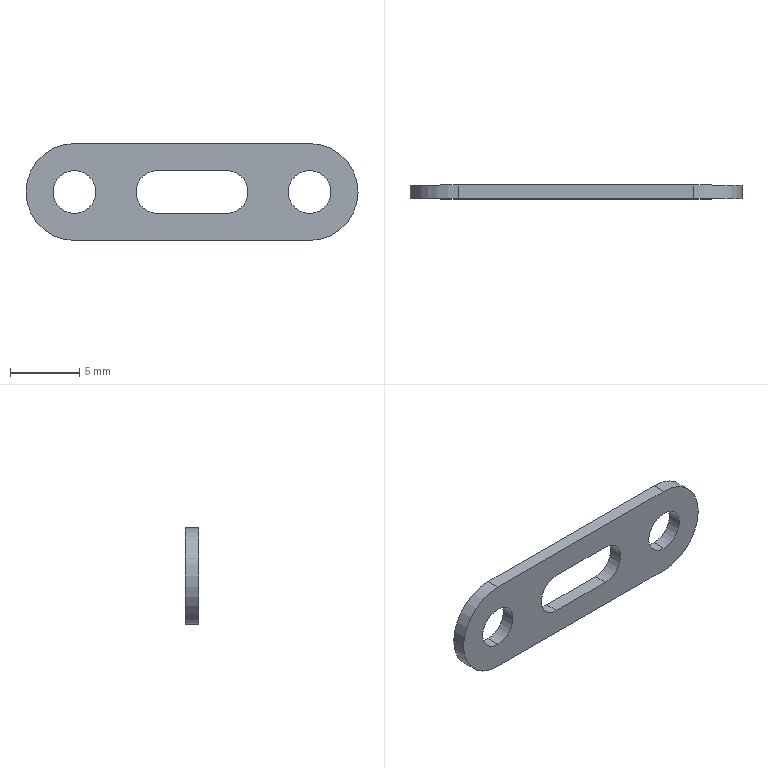Part | SolidWorks | features Extrusion 1 | 1 solid | 14 faces | box 23.98 x 1 x 7 mm | volume 119.201 mm3 | cylinder 8 | plane 6 | commonest cylinder face diameters 3.1 x6 7 x2
STEP:
#1=CARTESIAN_POINT('',(16.98,1.,-1.55));
#2=VERTEX_POINT('',#1);
#3=CARTESIAN_POINT('',(16.98,1.,1.55));
#4=VERTEX_POINT('',#3);
#5=CARTESIAN_POINT('',(16.98,1.,0.));
#6=DIRECTION('',(0.,1.,0.));
#7=DIRECTION('',(0.,0.,1.));
#8=AXIS2_PLACEMENT_3D('',#5,#6,#7);
#9=CIRCLE('',#8,1.55);
#10=EDGE_CURVE('',#2,#4,#9,.T.);
#11=ORIENTED_EDGE('',*,*,#10,.T.);
#12=CARTESIAN_POINT('',(16.98,0.,1.55));
#13=VERTEX_POINT('',#12);
#14=CARTESIAN_POINT('',(16.98,1.,1.55));
#15=DIRECTION('',(0.,-1.,0.));
#16=VECTOR('',#15,1000.);
#17=LINE('',#14,#16);
#18=EDGE_CURVE('',#4,#13,#17,.T.);
#19=ORIENTED_EDGE('',*,*,#18,.T.);
#20=CARTESIAN_POINT('',(16.98,0.,-1.55));
#21=VERTEX_POINT('',#20);
#22=CARTESIAN_POINT('',(16.98,0.,0.));
#23=DIRECTION('',(0.,1.,0.));
#24=DIRECTION('',(0.,0.,1.));
#25=AXIS2_PLACEMENT_3D('',#22,#23,#24);
#26=CIRCLE('',#25,1.55);
#27=EDGE_CURVE('',#21,#13,#26,.T.);
#28=ORIENTED_EDGE('',*,*,#27,.F.);
#29=CARTESIAN_POINT('',(16.98,1.,-1.55));
#30=DIRECTION('',(0.,-1.,0.));
#31=VECTOR('',#30,1000.);
#32=LINE('',#29,#31);
#33=EDGE_CURVE('',#2,#21,#32,.T.);
#34=ORIENTED_EDGE('',*,*,#33,.F.);
#35=EDGE_LOOP('',(#11,#19,#28,#34));
#36=FACE_OUTER_BOUND('',#35,.T.);
#37=CARTESIAN_POINT('',(16.98,1.,0.));
#38=DIRECTION('',(0.,-1.,0.));
#39=DIRECTION('',(0.,0.,-1.));
#40=AXIS2_PLACEMENT_3D('',#37,#38,#39);
#41=CYLINDRICAL_SURFACE('',#40,1.55);
#42=ADVANCED_FACE('',(#36),#41,.F.);
#43=CARTESIAN_POINT('',(0.,1.,-1.55));
#44=VERTEX_POINT('',#43);
#45=CARTESIAN_POINT('',(0.,1.,1.55));
#46=VERTEX_POINT('',#45);
#47=CARTESIAN_POINT('',(0.,1.,0.));
#48=DIRECTION('',(0.,1.,0.));
#49=DIRECTION('',(0.,0.,1.));
#50=AXIS2_PLACEMENT_3D('',#47,#48,#49);
#51=CIRCLE('',#50,1.55);
#52=EDGE_CURVE('',#44,#46,#51,.T.);
#53=ORIENTED_EDGE('',*,*,#52,.T.);
#54=CARTESIAN_POINT('',(0.,0.,1.55));
#55=VERTEX_POINT('',#54);
#56=CARTESIAN_POINT('',(0.,1.,1.55));
#57=DIRECTION('',(0.,-1.,0.));
#58=VECTOR('',#57,1000.);
#59=LINE('',#56,#58);
#60=EDGE_CURVE('',#46,#55,#59,.T.);
#61=ORIENTED_EDGE('',*,*,#60,.T.);
#62=CARTESIAN_POINT('',(0.,0.,-1.55));
#63=VERTEX_POINT('',#62);
#64=CARTESIAN_POINT('',(0.,0.,0.));
#65=DIRECTION('',(0.,1.,0.));
#66=DIRECTION('',(0.,0.,1.));
#67=AXIS2_PLACEMENT_3D('',#64,#65,#66);
#68=CIRCLE('',#67,1.55);
#69=EDGE_CURVE('',#63,#55,#68,.T.);
#70=ORIENTED_EDGE('',*,*,#69,.F.);
#71=CARTESIAN_POINT('',(0.,1.,-1.55));
#72=DIRECTION('',(0.,-1.,0.));
#73=VECTOR('',#72,1000.);
#74=LINE('',#71,#73);
#75=EDGE_CURVE('',#44,#63,#74,.T.);
#76=ORIENTED_EDGE('',*,*,#75,.F.);
#77=EDGE_LOOP('',(#53,#61,#70,#76));
#78=FACE_OUTER_BOUND('',#77,.T.);
#79=CARTESIAN_POINT('',(0.,1.,0.));
#80=DIRECTION('',(0.,-1.,0.));
#81=DIRECTION('',(0.,0.,-1.));
#82=AXIS2_PLACEMENT_3D('',#79,#80,#81);
#83=CYLINDRICAL_SURFACE('',#82,1.55);
#84=ADVANCED_FACE('',(#78),#83,.F.);
#85=CARTESIAN_POINT('',(10.99,0.,1.55));
#86=VERTEX_POINT('',#85);
#87=CARTESIAN_POINT('',(10.99,0.,-1.55));
#88=VERTEX_POINT('',#87);
#89=CARTESIAN_POINT('',(10.99,0.,0.));
#90=DIRECTION('',(0.,1.,0.));
#91=DIRECTION('',(0.,0.,1.));
#92=AXIS2_PLACEMENT_3D('',#89,#90,#91);
#93=CIRCLE('',#92,1.55);
#94=EDGE_CURVE('',#86,#88,#93,.T.);
#95=ORIENTED_EDGE('',*,*,#94,.F.);
#96=CARTESIAN_POINT('',(10.99,1.,1.55));
#97=VERTEX_POINT('',#96);
#98=CARTESIAN_POINT('',(10.99,1.,1.55));
#99=DIRECTION('',(0.,-1.,0.));
#100=VECTOR('',#99,1000.);
#101=LINE('',#98,#100);
#102=EDGE_CURVE('',#97,#86,#101,.T.);
#103=ORIENTED_EDGE('',*,*,#102,.F.);
#104=CARTESIAN_POINT('',(10.99,1.,-1.55));
#105=VERTEX_POINT('',#104);
#106=CARTESIAN_POINT('',(10.99,1.,0.));
#107=DIRECTION('',(0.,1.,0.));
#108=DIRECTION('',(0.,0.,1.));
#109=AXIS2_PLACEMENT_3D('',#106,#107,#108);
#110=CIRCLE('',#109,1.55);
#111=EDGE_CURVE('',#97,#105,#110,.T.);
#112=ORIENTED_EDGE('',*,*,#111,.T.);
#113=CARTESIAN_POINT('',(10.99,1.,-1.55));
#114=DIRECTION('',(0.,-1.,0.));
#115=VECTOR('',#114,1000.);
#116=LINE('',#113,#115);
#117=EDGE_CURVE('',#105,#88,#116,.T.);
#118=ORIENTED_EDGE('',*,*,#117,.T.);
#119=EDGE_LOOP('',(#95,#103,#112,#118));
#120=FACE_OUTER_BOUND('',#119,.T.);
#121=CARTESIAN_POINT('',(10.99,1.,0.));
#122=DIRECTION('',(0.,-1.,0.));
#123=DIRECTION('',(0.,0.,-1.));
#124=AXIS2_PLACEMENT_3D('',#121,#122,#123);
#125=CYLINDRICAL_SURFACE('',#124,1.55);
#126=ADVANCED_FACE('',(#120),#125,.F.);
#127=CARTESIAN_POINT('',(5.99,0.,1.55));
#128=VERTEX_POINT('',#127);
#129=CARTESIAN_POINT('',(0.,0.,1.55));
#130=DIRECTION('',(1.,0.,0.));
#131=VECTOR('',#130,1000.);
#132=LINE('',#129,#131);
#133=EDGE_CURVE('',#128,#86,#132,.T.);
#134=ORIENTED_EDGE('',*,*,#133,.F.);
#135=CARTESIAN_POINT('',(5.99,1.,1.55));
#136=VERTEX_POINT('',#135);
#137=CARTESIAN_POINT('',(5.99,1.,1.55));
#138=DIRECTION('',(0.,-1.,0.));
#139=VECTOR('',#138,1000.);
#140=LINE('',#137,#139);
#141=EDGE_CURVE('',#136,#128,#140,.T.);
#142=ORIENTED_EDGE('',*,*,#141,.F.);
#143=CARTESIAN_POINT('',(0.,1.,1.55));
#144=DIRECTION('',(1.,0.,0.));
#145=VECTOR('',#144,1000.);
#146=LINE('',#143,#145);
#147=EDGE_CURVE('',#136,#97,#146,.T.);
#148=ORIENTED_EDGE('',*,*,#147,.T.);
#149=ORIENTED_EDGE('',*,*,#102,.T.);
#150=EDGE_LOOP('',(#134,#142,#148,#149));
#151=FACE_OUTER_BOUND('',#150,.T.);
#152=CARTESIAN_POINT('',(0.,1.,1.55));
#153=DIRECTION('',(0.,0.,-1.));
#154=DIRECTION('',(-1.,0.,0.));
#155=AXIS2_PLACEMENT_3D('',#152,#153,#154);
#156=PLANE('',#155);
#157=ADVANCED_FACE('',(#151),#156,.T.);
#158=CARTESIAN_POINT('',(5.99,0.,-1.55));
#159=VERTEX_POINT('',#158);
#160=CARTESIAN_POINT('',(5.99,0.,0.));
#161=DIRECTION('',(0.,1.,0.));
#162=DIRECTION('',(0.,0.,1.));
#163=AXIS2_PLACEMENT_3D('',#160,#161,#162);
#164=CIRCLE('',#163,1.55);
#165=EDGE_CURVE('',#159,#128,#164,.T.);
#166=ORIENTED_EDGE('',*,*,#165,.F.);
#167=CARTESIAN_POINT('',(5.99,1.,-1.55));
#168=VERTEX_POINT('',#167);
#169=CARTESIAN_POINT('',(5.99,1.,-1.55));
#170=DIRECTION('',(0.,-1.,0.));
#171=VECTOR('',#170,1000.);
#172=LINE('',#169,#171);
#173=EDGE_CURVE('',#168,#159,#172,.T.);
#174=ORIENTED_EDGE('',*,*,#173,.F.);
#175=CARTESIAN_POINT('',(5.99,1.,0.));
#176=DIRECTION('',(0.,1.,0.));
#177=DIRECTION('',(0.,0.,1.));
#178=AXIS2_PLACEMENT_3D('',#175,#176,#177);
#179=CIRCLE('',#178,1.55);
#180=EDGE_CURVE('',#168,#136,#179,.T.);
#181=ORIENTED_EDGE('',*,*,#180,.T.);
#182=ORIENTED_EDGE('',*,*,#141,.T.);
#183=EDGE_LOOP('',(#166,#174,#181,#182));
#184=FACE_OUTER_BOUND('',#183,.T.);
#185=CARTESIAN_POINT('',(5.99,1.,0.));
#186=DIRECTION('',(0.,-1.,0.));
#187=DIRECTION('',(0.,0.,-1.));
#188=AXIS2_PLACEMENT_3D('',#185,#186,#187);
#189=CYLINDRICAL_SURFACE('',#188,1.55);
#190=ADVANCED_FACE('',(#184),#189,.F.);
#191=CARTESIAN_POINT('',(0.,0.,-3.5));
#192=VERTEX_POINT('',#191);
#193=CARTESIAN_POINT('',(0.,0.,3.5));
#194=VERTEX_POINT('',#193);
#195=CARTESIAN_POINT('',(0.,0.,0.));
#196=DIRECTION('',(0.,1.,0.));
#197=DIRECTION('',(0.,0.,1.));
#198=AXIS2_PLACEMENT_3D('',#195,#196,#197);
#199=CIRCLE('',#198,3.5);
#200=EDGE_CURVE('',#192,#194,#199,.T.);
#201=ORIENTED_EDGE('',*,*,#200,.T.);
#202=CARTESIAN_POINT('',(0.,1.,3.5));
#203=VERTEX_POINT('',#202);
#204=CARTESIAN_POINT('',(0.,1.,3.5));
#205=DIRECTION('',(0.,-1.,0.));
#206=VECTOR('',#205,1000.);
#207=LINE('',#204,#206);
#208=EDGE_CURVE('',#203,#194,#207,.T.);
#209=ORIENTED_EDGE('',*,*,#208,.F.);
#210=CARTESIAN_POINT('',(0.,1.,-3.5));
#211=VERTEX_POINT('',#210);
#212=CARTESIAN_POINT('',(0.,1.,0.));
#213=DIRECTION('',(0.,1.,0.));
#214=DIRECTION('',(0.,0.,1.));
#215=AXIS2_PLACEMENT_3D('',#212,#213,#214);
#216=CIRCLE('',#215,3.5);
#217=EDGE_CURVE('',#211,#203,#216,.T.);
#218=ORIENTED_EDGE('',*,*,#217,.F.);
#219=CARTESIAN_POINT('',(0.,1.,-3.5));
#220=DIRECTION('',(0.,-1.,0.));
#221=VECTOR('',#220,1000.);
#222=LINE('',#219,#221);
#223=EDGE_CURVE('',#211,#192,#222,.T.);
#224=ORIENTED_EDGE('',*,*,#223,.T.);
#225=EDGE_LOOP('',(#201,#209,#218,#224));
#226=FACE_OUTER_BOUND('',#225,.T.);
#227=CARTESIAN_POINT('',(0.,1.,0.));
#228=DIRECTION('',(0.,-1.,0.));
#229=DIRECTION('',(0.,0.,-1.));
#230=AXIS2_PLACEMENT_3D('',#227,#228,#229);
#231=CYLINDRICAL_SURFACE('',#230,3.5);
#232=ADVANCED_FACE('',(#226),#231,.T.);
#233=CARTESIAN_POINT('',(16.98,0.,3.5));
#234=VERTEX_POINT('',#233);
#235=CARTESIAN_POINT('',(0.,0.,3.5));
#236=DIRECTION('',(1.,0.,0.));
#237=VECTOR('',#236,1000.);
#238=LINE('',#235,#237);
#239=EDGE_CURVE('',#194,#234,#238,.T.);
#240=ORIENTED_EDGE('',*,*,#239,.T.);
#241=CARTESIAN_POINT('',(16.98,1.,3.5));
#242=VERTEX_POINT('',#241);
#243=CARTESIAN_POINT('',(16.98,1.,3.5));
#244=DIRECTION('',(0.,-1.,0.));
#245=VECTOR('',#244,1000.);
#246=LINE('',#243,#245);
#247=EDGE_CURVE('',#242,#234,#246,.T.);
#248=ORIENTED_EDGE('',*,*,#247,.F.);
#249=CARTESIAN_POINT('',(0.,1.,3.5));
#250=DIRECTION('',(1.,0.,0.));
#251=VECTOR('',#250,1000.);
#252=LINE('',#249,#251);
#253=EDGE_CURVE('',#203,#242,#252,.T.);
#254=ORIENTED_EDGE('',*,*,#253,.F.);
#255=ORIENTED_EDGE('',*,*,#208,.T.);
#256=EDGE_LOOP('',(#240,#248,#254,#255));
#257=FACE_OUTER_BOUND('',#256,.T.);
#258=CARTESIAN_POINT('',(0.,1.,3.5));
#259=DIRECTION('',(0.,0.,-1.));
#260=DIRECTION('',(-1.,0.,0.));
#261=AXIS2_PLACEMENT_3D('',#258,#259,#260);
#262=PLANE('',#261);
#263=ADVANCED_FACE('',(#257),#262,.F.);
#264=CARTESIAN_POINT('',(16.98,0.,-3.5));
#265=VERTEX_POINT('',#264);
#266=CARTESIAN_POINT('',(16.98,0.,0.));
#267=DIRECTION('',(0.,1.,0.));
#268=DIRECTION('',(0.,0.,1.));
#269=AXIS2_PLACEMENT_3D('',#266,#267,#268);
#270=CIRCLE('',#269,3.5);
#271=EDGE_CURVE('',#234,#265,#270,.T.);
#272=ORIENTED_EDGE('',*,*,#271,.T.);
#273=CARTESIAN_POINT('',(16.98,1.,-3.5));
#274=VERTEX_POINT('',#273);
#275=CARTESIAN_POINT('',(16.98,1.,-3.5));
#276=DIRECTION('',(0.,-1.,0.));
#277=VECTOR('',#276,1000.);
#278=LINE('',#275,#277);
#279=EDGE_CURVE('',#274,#265,#278,.T.);
#280=ORIENTED_EDGE('',*,*,#279,.F.);
#281=CARTESIAN_POINT('',(16.98,1.,0.));
#282=DIRECTION('',(0.,1.,0.));
#283=DIRECTION('',(0.,0.,1.));
#284=AXIS2_PLACEMENT_3D('',#281,#282,#283);
#285=CIRCLE('',#284,3.5);
#286=EDGE_CURVE('',#242,#274,#285,.T.);
#287=ORIENTED_EDGE('',*,*,#286,.F.);
#288=ORIENTED_EDGE('',*,*,#247,.T.);
#289=EDGE_LOOP('',(#272,#280,#287,#288));
#290=FACE_OUTER_BOUND('',#289,.T.);
#291=CARTESIAN_POINT('',(16.98,1.,0.));
#292=DIRECTION('',(0.,-1.,0.));
#293=DIRECTION('',(0.,0.,-1.));
#294=AXIS2_PLACEMENT_3D('',#291,#292,#293);
#295=CYLINDRICAL_SURFACE('',#294,3.5);
#296=ADVANCED_FACE('',(#290),#295,.T.);
#297=CARTESIAN_POINT('',(0.,0.,-1.55));
#298=DIRECTION('',(1.,0.,0.));
#299=VECTOR('',#298,1000.);
#300=LINE('',#297,#299);
#301=EDGE_CURVE('',#159,#88,#300,.T.);
#302=ORIENTED_EDGE('',*,*,#301,.T.);
#303=ORIENTED_EDGE('',*,*,#117,.F.);
#304=CARTESIAN_POINT('',(0.,1.,-1.55));
#305=DIRECTION('',(1.,0.,0.));
#306=VECTOR('',#305,1000.);
#307=LINE('',#304,#306);
#308=EDGE_CURVE('',#168,#105,#307,.T.);
#309=ORIENTED_EDGE('',*,*,#308,.F.);
#310=ORIENTED_EDGE('',*,*,#173,.T.);
#311=EDGE_LOOP('',(#302,#303,#309,#310));
#312=FACE_OUTER_BOUND('',#311,.T.);
#313=CARTESIAN_POINT('',(0.,1.,-1.55));
#314=DIRECTION('',(0.,0.,-1.));
#315=DIRECTION('',(-1.,0.,0.));
#316=AXIS2_PLACEMENT_3D('',#313,#314,#315);
#317=PLANE('',#316);
#318=ADVANCED_FACE('',(#312),#317,.F.);
#319=CARTESIAN_POINT('',(0.,0.,-3.5));
#320=DIRECTION('',(1.,0.,0.));
#321=VECTOR('',#320,1000.);
#322=LINE('',#319,#321);
#323=EDGE_CURVE('',#192,#265,#322,.T.);
#324=ORIENTED_EDGE('',*,*,#323,.F.);
#325=ORIENTED_EDGE('',*,*,#223,.F.);
#326=CARTESIAN_POINT('',(0.,1.,-3.5));
#327=DIRECTION('',(1.,0.,0.));
#328=VECTOR('',#327,1000.);
#329=LINE('',#326,#328);
#330=EDGE_CURVE('',#211,#274,#329,.T.);
#331=ORIENTED_EDGE('',*,*,#330,.T.);
#332=ORIENTED_EDGE('',*,*,#279,.T.);
#333=EDGE_LOOP('',(#324,#325,#331,#332));
#334=FACE_OUTER_BOUND('',#333,.T.);
#335=CARTESIAN_POINT('',(0.,1.,-3.5));
#336=DIRECTION('',(0.,0.,-1.));
#337=DIRECTION('',(-1.,0.,0.));
#338=AXIS2_PLACEMENT_3D('',#335,#336,#337);
#339=PLANE('',#338);
#340=ADVANCED_FACE('',(#334),#339,.T.);
#341=ORIENTED_EDGE('',*,*,#60,.F.);
#342=CARTESIAN_POINT('',(0.,1.,0.));
#343=DIRECTION('',(0.,1.,0.));
#344=DIRECTION('',(0.,0.,1.));
#345=AXIS2_PLACEMENT_3D('',#342,#343,#344);
#346=CIRCLE('',#345,1.55);
#347=EDGE_CURVE('',#46,#44,#346,.T.);
#348=ORIENTED_EDGE('',*,*,#347,.T.);
#349=ORIENTED_EDGE('',*,*,#75,.T.);
#350=CARTESIAN_POINT('',(0.,0.,0.));
#351=DIRECTION('',(0.,1.,0.));
#352=DIRECTION('',(0.,0.,1.));
#353=AXIS2_PLACEMENT_3D('',#350,#351,#352);
#354=CIRCLE('',#353,1.55);
#355=EDGE_CURVE('',#55,#63,#354,.T.);
#356=ORIENTED_EDGE('',*,*,#355,.F.);
#357=EDGE_LOOP('',(#341,#348,#349,#356));
#358=FACE_OUTER_BOUND('',#357,.T.);
#359=CARTESIAN_POINT('',(0.,1.,0.));
#360=DIRECTION('',(0.,-1.,0.));
#361=DIRECTION('',(0.,0.,-1.));
#362=AXIS2_PLACEMENT_3D('',#359,#360,#361);
#363=CYLINDRICAL_SURFACE('',#362,1.55);
#364=ADVANCED_FACE('',(#358),#363,.F.);
#365=ORIENTED_EDGE('',*,*,#18,.F.);
#366=CARTESIAN_POINT('',(16.98,1.,0.));
#367=DIRECTION('',(0.,1.,0.));
#368=DIRECTION('',(0.,0.,1.));
#369=AXIS2_PLACEMENT_3D('',#366,#367,#368);
#370=CIRCLE('',#369,1.55);
#371=EDGE_CURVE('',#4,#2,#370,.T.);
#372=ORIENTED_EDGE('',*,*,#371,.T.);
#373=ORIENTED_EDGE('',*,*,#33,.T.);
#374=CARTESIAN_POINT('',(16.98,0.,0.));
#375=DIRECTION('',(0.,1.,0.));
#376=DIRECTION('',(0.,0.,1.));
#377=AXIS2_PLACEMENT_3D('',#374,#375,#376);
#378=CIRCLE('',#377,1.55);
#379=EDGE_CURVE('',#13,#21,#378,.T.);
#380=ORIENTED_EDGE('',*,*,#379,.F.);
#381=EDGE_LOOP('',(#365,#372,#373,#380));
#382=FACE_OUTER_BOUND('',#381,.T.);
#383=CARTESIAN_POINT('',(16.98,1.,0.));
#384=DIRECTION('',(0.,-1.,0.));
#385=DIRECTION('',(0.,0.,-1.));
#386=AXIS2_PLACEMENT_3D('',#383,#384,#385);
#387=CYLINDRICAL_SURFACE('',#386,1.55);
#388=ADVANCED_FACE('',(#382),#387,.F.);
#389=ORIENTED_EDGE('',*,*,#52,.F.);
#390=ORIENTED_EDGE('',*,*,#347,.F.);
#391=EDGE_LOOP('',(#389,#390));
#392=FACE_BOUND('',#391,.T.);
#393=ORIENTED_EDGE('',*,*,#217,.T.);
#394=ORIENTED_EDGE('',*,*,#253,.T.);
#395=ORIENTED_EDGE('',*,*,#286,.T.);
#396=ORIENTED_EDGE('',*,*,#330,.F.);
#397=EDGE_LOOP('',(#393,#394,#395,#396));
#398=FACE_OUTER_BOUND('',#397,.T.);
#399=ORIENTED_EDGE('',*,*,#111,.F.);
#400=ORIENTED_EDGE('',*,*,#147,.F.);
#401=ORIENTED_EDGE('',*,*,#180,.F.);
#402=ORIENTED_EDGE('',*,*,#308,.T.);
#403=EDGE_LOOP('',(#399,#400,#401,#402));
#404=FACE_BOUND('',#403,.T.);
#405=ORIENTED_EDGE('',*,*,#10,.F.);
#406=ORIENTED_EDGE('',*,*,#371,.F.);
#407=EDGE_LOOP('',(#405,#406));
#408=FACE_BOUND('',#407,.T.);
#409=CARTESIAN_POINT('',(0.,1.,0.));
#410=DIRECTION('',(0.,1.,0.));
#411=DIRECTION('',(0.,0.,1.));
#412=AXIS2_PLACEMENT_3D('',#409,#410,#411);
#413=PLANE('',#412);
#414=ADVANCED_FACE('',(#392,#398,#404,#408),#413,.T.);
#415=ORIENTED_EDGE('',*,*,#69,.T.);
#416=ORIENTED_EDGE('',*,*,#355,.T.);
#417=EDGE_LOOP('',(#415,#416));
#418=FACE_BOUND('',#417,.T.);
#419=ORIENTED_EDGE('',*,*,#200,.F.);
#420=ORIENTED_EDGE('',*,*,#323,.T.);
#421=ORIENTED_EDGE('',*,*,#271,.F.);
#422=ORIENTED_EDGE('',*,*,#239,.F.);
#423=EDGE_LOOP('',(#419,#420,#421,#422));
#424=FACE_OUTER_BOUND('',#423,.T.);
#425=ORIENTED_EDGE('',*,*,#94,.T.);
#426=ORIENTED_EDGE('',*,*,#301,.F.);
#427=ORIENTED_EDGE('',*,*,#165,.T.);
#428=ORIENTED_EDGE('',*,*,#133,.T.);
#429=EDGE_LOOP('',(#425,#426,#427,#428));
#430=FACE_BOUND('',#429,.T.);
#431=ORIENTED_EDGE('',*,*,#27,.T.);
#432=ORIENTED_EDGE('',*,*,#379,.T.);
#433=EDGE_LOOP('',(#431,#432));
#434=FACE_BOUND('',#433,.T.);
#435=CARTESIAN_POINT('',(0.,0.,0.));
#436=DIRECTION('',(0.,1.,0.));
#437=DIRECTION('',(0.,0.,1.));
#438=AXIS2_PLACEMENT_3D('',#435,#436,#437);
#439=PLANE('',#438);
#440=ADVANCED_FACE('',(#418,#424,#430,#434),#439,.F.);
#441=CLOSED_SHELL('',(#42,#84,#126,#157,#190,#232,#263,#296,#318,#340,#364,#388,#414,#440));
#442=MANIFOLD_SOLID_BREP('',#441);
#443=CARTESIAN_POINT('',(0.,0.,0.));
#444=DIRECTION('',(0.,0.,1.));
#445=DIRECTION('',(1.,0.,0.));
#446=AXIS2_PLACEMENT_3D('',#443,#444,#445);
#447=(LENGTH_UNIT()NAMED_UNIT(*)SI_UNIT(.MILLI.,.METRE.));
#448=UNCERTAINTY_MEASURE_WITH_UNIT(LENGTH_MEASURE(0.00001),#447,'','');
#449=(NAMED_UNIT(*)PLANE_ANGLE_UNIT()SI_UNIT($,.RADIAN.));
#450=(NAMED_UNIT(*)SI_UNIT($,.STERADIAN.)SOLID_ANGLE_UNIT());
#451=(GEOMETRIC_REPRESENTATION_CONTEXT(3)GLOBAL_UNCERTAINTY_ASSIGNED_CONTEXT((#448))GLOBAL_UNIT_ASSIGNED_CONTEXT((#447,#449,#450))REPRESENTATION_CONTEXT('',''));
#452=ADVANCED_BREP_SHAPE_REPRESENTATION('',(#442,#446),#451);